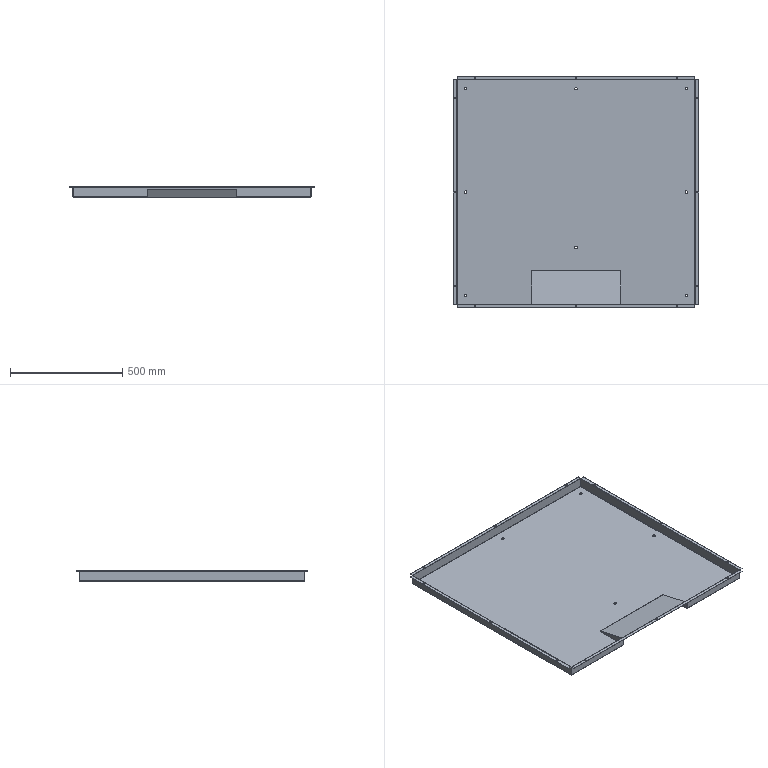Part | SolidWorks | 2 solids | 170 faces | box 1095 x 1035 x 45 mm | volume 1302233 mm3 | plane 90 | cylinder 68 | spline 12 | commonest cylinder face diameters 7 x30 11 x16 0.4 x9 2.4 x9 2 x2 4 x2